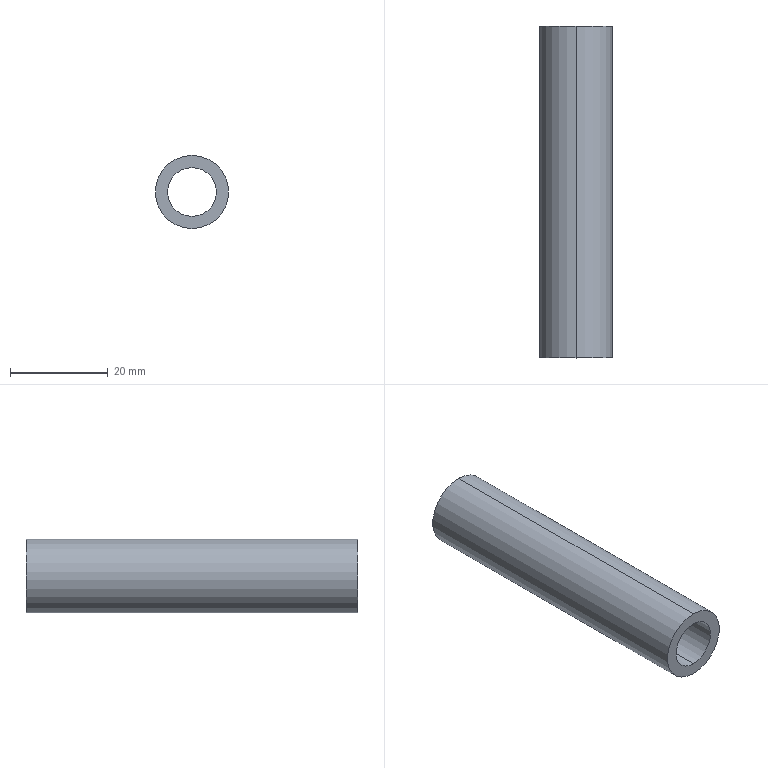Part | STEP file | 1 solid | 6 faces | box 15 x 68 x 15 mm | volume 6676 mm3 | cylinder 4 | plane 2 | commonest cylinder face diameters 10 x2 15 x2
STEP:
#1=CARTESIAN_POINT('',(0.,0.,0.));
#2=DIRECTION('',(0.,0.,1.));
#3=DIRECTION('',(1.,0.,0.));
#4=AXIS2_PLACEMENT_3D('',#1,#2,#3);
#5=CARTESIAN_POINT('',(0.,0.,7.5));
#6=VERTEX_POINT('',#5);
#7=CARTESIAN_POINT('',(0.,0.,-7.5));
#8=VERTEX_POINT('',#7);
#9=CARTESIAN_POINT('',(0.,0.,0.));
#10=DIRECTION('',(0.,1.,0.));
#11=DIRECTION('',(0.,0.,1.));
#12=AXIS2_PLACEMENT_3D('',#9,#10,#11);
#13=CIRCLE('',#12,7.5);
#14=CARTESIAN_POINT('',(0.,0.,0.));
#15=DIRECTION('',(0.,1.,0.));
#16=DIRECTION('',(0.,0.,1.));
#17=AXIS2_PLACEMENT_3D('',#14,#15,#16);
#18=CYLINDRICAL_SURFACE('',#17,7.5);
#19=CARTESIAN_POINT('',(0.,0.));
#20=DIRECTION('',(1.,0.));
#21=VECTOR('',#20,1.);
#22=LINE('',#19,#21);
#23=(GEOMETRIC_REPRESENTATION_CONTEXT(2)PARAMETRIC_REPRESENTATION_CONTEXT()REPRESENTATION_CONTEXT('',''));
#24=DEFINITIONAL_REPRESENTATION('',(#22),#23);
#25=PCURVE('',#18,#24);
#26=CARTESIAN_POINT('',(0.,0.,0.));
#27=DIRECTION('',(0.,1.,0.));
#28=DIRECTION('',(0.,0.,1.));
#29=AXIS2_PLACEMENT_3D('',#26,#27,#28);
#30=PLANE('',#29);
#31=CARTESIAN_POINT('',(0.,0.));
#32=DIRECTION('',(1.,0.));
#33=AXIS2_PLACEMENT_2D('',#31,#32);
#34=CIRCLE('',#33,7.5);
#35=(GEOMETRIC_REPRESENTATION_CONTEXT(2)PARAMETRIC_REPRESENTATION_CONTEXT()REPRESENTATION_CONTEXT('',''));
#36=DEFINITIONAL_REPRESENTATION('',(#34),#35);
#37=PCURVE('',#30,#36);
#38=SURFACE_CURVE('',#13,(#25,#37),.PCURVE_S1.);
#39=EDGE_CURVE('',#6,#8,#38,.T.);
#40=ORIENTED_EDGE('',*,*,#39,.T.);
#41=CARTESIAN_POINT('',(0.,68.,-7.5));
#42=VERTEX_POINT('',#41);
#43=CARTESIAN_POINT('',(0.,0.,-7.5));
#44=DIRECTION('',(0.,1.,0.));
#45=VECTOR('',#44,1.);
#46=LINE('',#43,#45);
#47=CARTESIAN_POINT('',(3.142,0.));
#48=DIRECTION('',(0.,1.));
#49=VECTOR('',#48,1.);
#50=LINE('',#47,#49);
#51=(GEOMETRIC_REPRESENTATION_CONTEXT(2)PARAMETRIC_REPRESENTATION_CONTEXT()REPRESENTATION_CONTEXT('',''));
#52=DEFINITIONAL_REPRESENTATION('',(#50),#51);
#53=PCURVE('',#18,#52);
#54=CARTESIAN_POINT('',(0.,0.,0.));
#55=DIRECTION('',(0.,1.,0.));
#56=DIRECTION('',(0.,0.,1.));
#57=AXIS2_PLACEMENT_3D('',#54,#55,#56);
#58=CYLINDRICAL_SURFACE('',#57,7.5);
#59=CARTESIAN_POINT('',(3.142,0.));
#60=DIRECTION('',(0.,1.));
#61=VECTOR('',#60,1.);
#62=LINE('',#59,#61);
#63=(GEOMETRIC_REPRESENTATION_CONTEXT(2)PARAMETRIC_REPRESENTATION_CONTEXT()REPRESENTATION_CONTEXT('',''));
#64=DEFINITIONAL_REPRESENTATION('',(#62),#63);
#65=PCURVE('',#58,#64);
#66=SURFACE_CURVE('',#46,(#53,#65),.PCURVE_S1.);
#67=EDGE_CURVE('',#8,#42,#66,.T.);
#68=ORIENTED_EDGE('',*,*,#67,.T.);
#69=CARTESIAN_POINT('',(0.,68.,7.5));
#70=VERTEX_POINT('',#69);
#71=CARTESIAN_POINT('',(0.,68.,0.));
#72=DIRECTION('',(0.,-1.,0.));
#73=DIRECTION('',(0.,0.,1.));
#74=AXIS2_PLACEMENT_3D('',#71,#72,#73);
#75=CIRCLE('',#74,7.5);
#76=CARTESIAN_POINT('',(6.283,68.));
#77=DIRECTION('',(-1.,0.));
#78=VECTOR('',#77,1.);
#79=LINE('',#76,#78);
#80=(GEOMETRIC_REPRESENTATION_CONTEXT(2)PARAMETRIC_REPRESENTATION_CONTEXT()REPRESENTATION_CONTEXT('',''));
#81=DEFINITIONAL_REPRESENTATION('',(#79),#80);
#82=PCURVE('',#18,#81);
#83=CARTESIAN_POINT('',(0.,68.,0.));
#84=DIRECTION('',(0.,1.,0.));
#85=DIRECTION('',(0.,0.,1.));
#86=AXIS2_PLACEMENT_3D('',#83,#84,#85);
#87=PLANE('',#86);
#88=CARTESIAN_POINT('',(7.5,0.));
#89=CARTESIAN_POINT('',(7.5,-12.99));
#90=CARTESIAN_POINT('',(-3.75,-6.495));
#91=CARTESIAN_POINT('',(-15.,0.));
#92=CARTESIAN_POINT('',(-3.75,6.495));
#93=CARTESIAN_POINT('',(7.5,12.99));
#94=CARTESIAN_POINT('',(7.5,0.));
#95=(BOUNDED_CURVE()B_SPLINE_CURVE(2,(#88,#89,#90,#91,#92,#93,#94),.UNSPECIFIED.,.T.,.F.)B_SPLINE_CURVE_WITH_KNOTS((1,2,2,2,2,1),(-2.094,0.,2.094,4.189,6.283,8.378),.UNSPECIFIED.)CURVE()GEOMETRIC_REPRESENTATION_ITEM()RATIONAL_B_SPLINE_CURVE((1.,0.5,1.,0.5,1.,0.5,1.))REPRESENTATION_ITEM(''));
#96=(GEOMETRIC_REPRESENTATION_CONTEXT(2)PARAMETRIC_REPRESENTATION_CONTEXT()REPRESENTATION_CONTEXT('',''));
#97=DEFINITIONAL_REPRESENTATION('',(#95),#96);
#98=PCURVE('',#87,#97);
#99=SURFACE_CURVE('',#75,(#82,#98),.PCURVE_S1.);
#100=EDGE_CURVE('',#42,#70,#99,.T.);
#101=ORIENTED_EDGE('',*,*,#100,.T.);
#102=CARTESIAN_POINT('',(0.,0.,7.5));
#103=DIRECTION('',(0.,1.,0.));
#104=VECTOR('',#103,1.);
#105=LINE('',#102,#104);
#106=CARTESIAN_POINT('',(0.,0.));
#107=DIRECTION('',(0.,1.));
#108=VECTOR('',#107,1.);
#109=LINE('',#106,#108);
#110=(GEOMETRIC_REPRESENTATION_CONTEXT(2)PARAMETRIC_REPRESENTATION_CONTEXT()REPRESENTATION_CONTEXT('',''));
#111=DEFINITIONAL_REPRESENTATION('',(#109),#110);
#112=PCURVE('',#18,#111);
#113=CARTESIAN_POINT('',(6.283,0.));
#114=DIRECTION('',(0.,1.));
#115=VECTOR('',#114,1.);
#116=LINE('',#113,#115);
#117=(GEOMETRIC_REPRESENTATION_CONTEXT(2)PARAMETRIC_REPRESENTATION_CONTEXT()REPRESENTATION_CONTEXT('',''));
#118=DEFINITIONAL_REPRESENTATION('',(#116),#117);
#119=PCURVE('',#58,#118);
#120=SURFACE_CURVE('',#105,(#112,#119),.PCURVE_S1.);
#121=EDGE_CURVE('',#6,#70,#120,.T.);
#122=ORIENTED_EDGE('',*,*,#121,.F.);
#123=EDGE_LOOP('',(#40,#68,#101,#122));
#124=FACE_BOUND('',#123,.T.);
#125=ADVANCED_FACE('',(#124),#18,.T.);
#126=CARTESIAN_POINT('',(0.,0.,5.));
#127=VERTEX_POINT('',#126);
#128=CARTESIAN_POINT('',(0.,68.,5.));
#129=VERTEX_POINT('',#128);
#130=CARTESIAN_POINT('',(0.,0.,5.));
#131=DIRECTION('',(0.,1.,0.));
#132=VECTOR('',#131,1.);
#133=LINE('',#130,#132);
#134=CARTESIAN_POINT('',(0.,0.,0.));
#135=DIRECTION('',(0.,1.,0.));
#136=DIRECTION('',(0.,0.,1.));
#137=AXIS2_PLACEMENT_3D('',#134,#135,#136);
#138=CYLINDRICAL_SURFACE('',#137,5.);
#139=CARTESIAN_POINT('',(6.283,0.));
#140=DIRECTION('',(0.,1.));
#141=VECTOR('',#140,1.);
#142=LINE('',#139,#141);
#143=(GEOMETRIC_REPRESENTATION_CONTEXT(2)PARAMETRIC_REPRESENTATION_CONTEXT()REPRESENTATION_CONTEXT('',''));
#144=DEFINITIONAL_REPRESENTATION('',(#142),#143);
#145=PCURVE('',#138,#144);
#146=CARTESIAN_POINT('',(0.,0.,0.));
#147=DIRECTION('',(0.,1.,0.));
#148=DIRECTION('',(0.,0.,1.));
#149=AXIS2_PLACEMENT_3D('',#146,#147,#148);
#150=CYLINDRICAL_SURFACE('',#149,5.);
#151=CARTESIAN_POINT('',(0.,0.));
#152=DIRECTION('',(0.,1.));
#153=VECTOR('',#152,1.);
#154=LINE('',#151,#153);
#155=(GEOMETRIC_REPRESENTATION_CONTEXT(2)PARAMETRIC_REPRESENTATION_CONTEXT()REPRESENTATION_CONTEXT('',''));
#156=DEFINITIONAL_REPRESENTATION('',(#154),#155);
#157=PCURVE('',#150,#156);
#158=SURFACE_CURVE('',#133,(#145,#157),.PCURVE_S1.);
#159=EDGE_CURVE('',#127,#129,#158,.T.);
#160=ORIENTED_EDGE('',*,*,#159,.T.);
#161=CARTESIAN_POINT('',(0.,68.,-5.));
#162=VERTEX_POINT('',#161);
#163=CARTESIAN_POINT('',(0.,68.,0.));
#164=DIRECTION('',(0.,-1.,0.));
#165=DIRECTION('',(0.,0.,1.));
#166=AXIS2_PLACEMENT_3D('',#163,#164,#165);
#167=CIRCLE('',#166,5.);
#168=CARTESIAN_POINT('',(6.283,68.));
#169=DIRECTION('',(-1.,0.));
#170=VECTOR('',#169,1.);
#171=LINE('',#168,#170);
#172=(GEOMETRIC_REPRESENTATION_CONTEXT(2)PARAMETRIC_REPRESENTATION_CONTEXT()REPRESENTATION_CONTEXT('',''));
#173=DEFINITIONAL_REPRESENTATION('',(#171),#172);
#174=PCURVE('',#138,#173);
#175=CARTESIAN_POINT('',(5.,0.));
#176=CARTESIAN_POINT('',(5.,-8.66));
#177=CARTESIAN_POINT('',(-2.5,-4.33));
#178=CARTESIAN_POINT('',(-10.,0.));
#179=CARTESIAN_POINT('',(-2.5,4.33));
#180=CARTESIAN_POINT('',(5.,8.66));
#181=CARTESIAN_POINT('',(5.,0.));
#182=(BOUNDED_CURVE()B_SPLINE_CURVE(2,(#175,#176,#177,#178,#179,#180,#181),.UNSPECIFIED.,.T.,.F.)B_SPLINE_CURVE_WITH_KNOTS((1,2,2,2,2,1),(-2.094,0.,2.094,4.189,6.283,8.378),.UNSPECIFIED.)CURVE()GEOMETRIC_REPRESENTATION_ITEM()RATIONAL_B_SPLINE_CURVE((1.,0.5,1.,0.5,1.,0.5,1.))REPRESENTATION_ITEM(''));
#183=(GEOMETRIC_REPRESENTATION_CONTEXT(2)PARAMETRIC_REPRESENTATION_CONTEXT()REPRESENTATION_CONTEXT('',''));
#184=DEFINITIONAL_REPRESENTATION('',(#182),#183);
#185=PCURVE('',#87,#184);
#186=SURFACE_CURVE('',#167,(#174,#185),.PCURVE_S1.);
#187=EDGE_CURVE('',#129,#162,#186,.T.);
#188=ORIENTED_EDGE('',*,*,#187,.T.);
#189=CARTESIAN_POINT('',(0.,0.,-5.));
#190=VERTEX_POINT('',#189);
#191=CARTESIAN_POINT('',(0.,0.,-5.));
#192=DIRECTION('',(0.,1.,0.));
#193=VECTOR('',#192,1.);
#194=LINE('',#191,#193);
#195=CARTESIAN_POINT('',(3.142,0.));
#196=DIRECTION('',(0.,1.));
#197=VECTOR('',#196,1.);
#198=LINE('',#195,#197);
#199=(GEOMETRIC_REPRESENTATION_CONTEXT(2)PARAMETRIC_REPRESENTATION_CONTEXT()REPRESENTATION_CONTEXT('',''));
#200=DEFINITIONAL_REPRESENTATION('',(#198),#199);
#201=PCURVE('',#138,#200);
#202=CARTESIAN_POINT('',(3.142,0.));
#203=DIRECTION('',(0.,1.));
#204=VECTOR('',#203,1.);
#205=LINE('',#202,#204);
#206=(GEOMETRIC_REPRESENTATION_CONTEXT(2)PARAMETRIC_REPRESENTATION_CONTEXT()REPRESENTATION_CONTEXT('',''));
#207=DEFINITIONAL_REPRESENTATION('',(#205),#206);
#208=PCURVE('',#150,#207);
#209=SURFACE_CURVE('',#194,(#201,#208),.PCURVE_S1.);
#210=EDGE_CURVE('',#190,#162,#209,.T.);
#211=ORIENTED_EDGE('',*,*,#210,.F.);
#212=CARTESIAN_POINT('',(0.,0.,0.));
#213=DIRECTION('',(0.,-1.,0.));
#214=DIRECTION('',(0.,0.,1.));
#215=AXIS2_PLACEMENT_3D('',#212,#213,#214);
#216=CIRCLE('',#215,5.);
#217=CARTESIAN_POINT('',(6.283,0.));
#218=DIRECTION('',(-1.,0.));
#219=VECTOR('',#218,1.);
#220=LINE('',#217,#219);
#221=(GEOMETRIC_REPRESENTATION_CONTEXT(2)PARAMETRIC_REPRESENTATION_CONTEXT()REPRESENTATION_CONTEXT('',''));
#222=DEFINITIONAL_REPRESENTATION('',(#220),#221);
#223=PCURVE('',#138,#222);
#224=CARTESIAN_POINT('',(5.,0.));
#225=CARTESIAN_POINT('',(5.,-8.66));
#226=CARTESIAN_POINT('',(-2.5,-4.33));
#227=CARTESIAN_POINT('',(-10.,0.));
#228=CARTESIAN_POINT('',(-2.5,4.33));
#229=CARTESIAN_POINT('',(5.,8.66));
#230=CARTESIAN_POINT('',(5.,0.));
#231=(BOUNDED_CURVE()B_SPLINE_CURVE(2,(#224,#225,#226,#227,#228,#229,#230),.UNSPECIFIED.,.T.,.F.)B_SPLINE_CURVE_WITH_KNOTS((1,2,2,2,2,1),(-2.094,0.,2.094,4.189,6.283,8.378),.UNSPECIFIED.)CURVE()GEOMETRIC_REPRESENTATION_ITEM()RATIONAL_B_SPLINE_CURVE((1.,0.5,1.,0.5,1.,0.5,1.))REPRESENTATION_ITEM(''));
#232=(GEOMETRIC_REPRESENTATION_CONTEXT(2)PARAMETRIC_REPRESENTATION_CONTEXT()REPRESENTATION_CONTEXT('',''));
#233=DEFINITIONAL_REPRESENTATION('',(#231),#232);
#234=PCURVE('',#30,#233);
#235=SURFACE_CURVE('',#216,(#223,#234),.PCURVE_S1.);
#236=EDGE_CURVE('',#127,#190,#235,.T.);
#237=ORIENTED_EDGE('',*,*,#236,.F.);
#238=EDGE_LOOP('',(#160,#188,#211,#237));
#239=FACE_BOUND('',#238,.F.);
#240=ADVANCED_FACE('',(#239),#138,.F.);
#241=ORIENTED_EDGE('',*,*,#67,.F.);
#242=CARTESIAN_POINT('',(0.,0.,0.));
#243=DIRECTION('',(0.,1.,0.));
#244=DIRECTION('',(0.,0.,1.));
#245=AXIS2_PLACEMENT_3D('',#242,#243,#244);
#246=CIRCLE('',#245,7.5);
#247=CARTESIAN_POINT('',(0.,0.));
#248=DIRECTION('',(1.,0.));
#249=VECTOR('',#248,1.);
#250=LINE('',#247,#249);
#251=(GEOMETRIC_REPRESENTATION_CONTEXT(2)PARAMETRIC_REPRESENTATION_CONTEXT()REPRESENTATION_CONTEXT('',''));
#252=DEFINITIONAL_REPRESENTATION('',(#250),#251);
#253=PCURVE('',#58,#252);
#254=CARTESIAN_POINT('',(0.,0.));
#255=DIRECTION('',(1.,0.));
#256=AXIS2_PLACEMENT_2D('',#254,#255);
#257=CIRCLE('',#256,7.5);
#258=(GEOMETRIC_REPRESENTATION_CONTEXT(2)PARAMETRIC_REPRESENTATION_CONTEXT()REPRESENTATION_CONTEXT('',''));
#259=DEFINITIONAL_REPRESENTATION('',(#257),#258);
#260=PCURVE('',#30,#259);
#261=SURFACE_CURVE('',#246,(#253,#260),.PCURVE_S1.);
#262=EDGE_CURVE('',#8,#6,#261,.T.);
#263=ORIENTED_EDGE('',*,*,#262,.T.);
#264=ORIENTED_EDGE('',*,*,#121,.T.);
#265=CARTESIAN_POINT('',(0.,68.,0.));
#266=DIRECTION('',(0.,-1.,0.));
#267=DIRECTION('',(0.,0.,1.));
#268=AXIS2_PLACEMENT_3D('',#265,#266,#267);
#269=CIRCLE('',#268,7.5);
#270=CARTESIAN_POINT('',(6.283,68.));
#271=DIRECTION('',(-1.,0.));
#272=VECTOR('',#271,1.);
#273=LINE('',#270,#272);
#274=(GEOMETRIC_REPRESENTATION_CONTEXT(2)PARAMETRIC_REPRESENTATION_CONTEXT()REPRESENTATION_CONTEXT('',''));
#275=DEFINITIONAL_REPRESENTATION('',(#273),#274);
#276=PCURVE('',#58,#275);
#277=CARTESIAN_POINT('',(7.5,0.));
#278=CARTESIAN_POINT('',(7.5,-12.99));
#279=CARTESIAN_POINT('',(-3.75,-6.495));
#280=CARTESIAN_POINT('',(-15.,0.));
#281=CARTESIAN_POINT('',(-3.75,6.495));
#282=CARTESIAN_POINT('',(7.5,12.99));
#283=CARTESIAN_POINT('',(7.5,0.));
#284=(BOUNDED_CURVE()B_SPLINE_CURVE(2,(#277,#278,#279,#280,#281,#282,#283),.UNSPECIFIED.,.T.,.F.)B_SPLINE_CURVE_WITH_KNOTS((1,2,2,2,2,1),(-2.094,0.,2.094,4.189,6.283,8.378),.UNSPECIFIED.)CURVE()GEOMETRIC_REPRESENTATION_ITEM()RATIONAL_B_SPLINE_CURVE((1.,0.5,1.,0.5,1.,0.5,1.))REPRESENTATION_ITEM(''));
#285=(GEOMETRIC_REPRESENTATION_CONTEXT(2)PARAMETRIC_REPRESENTATION_CONTEXT()REPRESENTATION_CONTEXT('',''));
#286=DEFINITIONAL_REPRESENTATION('',(#284),#285);
#287=PCURVE('',#87,#286);
#288=SURFACE_CURVE('',#269,(#276,#287),.PCURVE_S1.);
#289=EDGE_CURVE('',#70,#42,#288,.T.);
#290=ORIENTED_EDGE('',*,*,#289,.T.);
#291=EDGE_LOOP('',(#241,#263,#264,#290));
#292=FACE_BOUND('',#291,.T.);
#293=ADVANCED_FACE('',(#292),#58,.T.);
#294=ORIENTED_EDGE('',*,*,#39,.F.);
#295=ORIENTED_EDGE('',*,*,#262,.F.);
#296=EDGE_LOOP('',(#294,#295));
#297=FACE_BOUND('',#296,.T.);
#298=ORIENTED_EDGE('',*,*,#236,.F.);
#299=CARTESIAN_POINT('',(0.,0.,0.));
#300=DIRECTION('',(0.,-1.,0.));
#301=DIRECTION('',(0.,0.,1.));
#302=AXIS2_PLACEMENT_3D('',#299,#300,#301);
#303=CIRCLE('',#302,5.);
#304=CARTESIAN_POINT('',(5.,0.));
#305=CARTESIAN_POINT('',(5.,-8.66));
#306=CARTESIAN_POINT('',(-2.5,-4.33));
#307=CARTESIAN_POINT('',(-10.,0.));
#308=CARTESIAN_POINT('',(-2.5,4.33));
#309=CARTESIAN_POINT('',(5.,8.66));
#310=CARTESIAN_POINT('',(5.,0.));
#311=(BOUNDED_CURVE()B_SPLINE_CURVE(2,(#304,#305,#306,#307,#308,#309,#310),.UNSPECIFIED.,.T.,.F.)B_SPLINE_CURVE_WITH_KNOTS((1,2,2,2,2,1),(-2.094,0.,2.094,4.189,6.283,8.378),.UNSPECIFIED.)CURVE()GEOMETRIC_REPRESENTATION_ITEM()RATIONAL_B_SPLINE_CURVE((1.,0.5,1.,0.5,1.,0.5,1.))REPRESENTATION_ITEM(''));
#312=(GEOMETRIC_REPRESENTATION_CONTEXT(2)PARAMETRIC_REPRESENTATION_CONTEXT()REPRESENTATION_CONTEXT('',''));
#313=DEFINITIONAL_REPRESENTATION('',(#311),#312);
#314=PCURVE('',#30,#313);
#315=CARTESIAN_POINT('',(6.283,0.));
#316=DIRECTION('',(-1.,0.));
#317=VECTOR('',#316,1.);
#318=LINE('',#315,#317);
#319=(GEOMETRIC_REPRESENTATION_CONTEXT(2)PARAMETRIC_REPRESENTATION_CONTEXT()REPRESENTATION_CONTEXT('',''));
#320=DEFINITIONAL_REPRESENTATION('',(#318),#319);
#321=PCURVE('',#150,#320);
#322=SURFACE_CURVE('',#303,(#314,#321),.PCURVE_S1.);
#323=EDGE_CURVE('',#190,#127,#322,.T.);
#324=ORIENTED_EDGE('',*,*,#323,.F.);
#325=EDGE_LOOP('',(#298,#324));
#326=FACE_BOUND('',#325,.T.);
#327=ADVANCED_FACE('',(#297,#326),#30,.F.);
#328=ORIENTED_EDGE('',*,*,#289,.F.);
#329=ORIENTED_EDGE('',*,*,#100,.F.);
#330=EDGE_LOOP('',(#328,#329));
#331=FACE_BOUND('',#330,.T.);
#332=ORIENTED_EDGE('',*,*,#187,.T.);
#333=CARTESIAN_POINT('',(0.,68.,0.));
#334=DIRECTION('',(0.,-1.,0.));
#335=DIRECTION('',(0.,0.,1.));
#336=AXIS2_PLACEMENT_3D('',#333,#334,#335);
#337=CIRCLE('',#336,5.);
#338=CARTESIAN_POINT('',(5.,0.));
#339=CARTESIAN_POINT('',(5.,-8.66));
#340=CARTESIAN_POINT('',(-2.5,-4.33));
#341=CARTESIAN_POINT('',(-10.,0.));
#342=CARTESIAN_POINT('',(-2.5,4.33));
#343=CARTESIAN_POINT('',(5.,8.66));
#344=CARTESIAN_POINT('',(5.,0.));
#345=(BOUNDED_CURVE()B_SPLINE_CURVE(2,(#338,#339,#340,#341,#342,#343,#344),.UNSPECIFIED.,.T.,.F.)B_SPLINE_CURVE_WITH_KNOTS((1,2,2,2,2,1),(-2.094,0.,2.094,4.189,6.283,8.378),.UNSPECIFIED.)CURVE()GEOMETRIC_REPRESENTATION_ITEM()RATIONAL_B_SPLINE_CURVE((1.,0.5,1.,0.5,1.,0.5,1.))REPRESENTATION_ITEM(''));
#346=(GEOMETRIC_REPRESENTATION_CONTEXT(2)PARAMETRIC_REPRESENTATION_CONTEXT()REPRESENTATION_CONTEXT('',''));
#347=DEFINITIONAL_REPRESENTATION('',(#345),#346);
#348=PCURVE('',#87,#347);
#349=CARTESIAN_POINT('',(6.283,68.));
#350=DIRECTION('',(-1.,0.));
#351=VECTOR('',#350,1.);
#352=LINE('',#349,#351);
#353=(GEOMETRIC_REPRESENTATION_CONTEXT(2)PARAMETRIC_REPRESENTATION_CONTEXT()REPRESENTATION_CONTEXT('',''));
#354=DEFINITIONAL_REPRESENTATION('',(#352),#353);
#355=PCURVE('',#150,#354);
#356=SURFACE_CURVE('',#337,(#348,#355),.PCURVE_S1.);
#357=EDGE_CURVE('',#162,#129,#356,.T.);
#358=ORIENTED_EDGE('',*,*,#357,.T.);
#359=EDGE_LOOP('',(#332,#358));
#360=FACE_BOUND('',#359,.T.);
#361=ADVANCED_FACE('',(#331,#360),#87,.T.);
#362=ORIENTED_EDGE('',*,*,#357,.T.);
#363=ORIENTED_EDGE('',*,*,#159,.F.);
#364=ORIENTED_EDGE('',*,*,#323,.F.);
#365=ORIENTED_EDGE('',*,*,#210,.T.);
#366=EDGE_LOOP('',(#362,#363,#364,#365));
#367=FACE_BOUND('',#366,.F.);
#368=ADVANCED_FACE('',(#367),#150,.F.);
#369=CLOSED_SHELL('',(#125,#240,#293,#327,#361,#368));
#370=MANIFOLD_SOLID_BREP('',#369);
#371=(LENGTH_UNIT()NAMED_UNIT(*)SI_UNIT(.MILLI.,.METRE.));
#372=UNCERTAINTY_MEASURE_WITH_UNIT(LENGTH_MEASURE(0.0000001),#371,'','');
#373=(NAMED_UNIT(*)PLANE_ANGLE_UNIT()SI_UNIT($,.RADIAN.));
#374=(NAMED_UNIT(*)SI_UNIT($,.STERADIAN.)SOLID_ANGLE_UNIT());
#375=(GEOMETRIC_REPRESENTATION_CONTEXT(3)GLOBAL_UNCERTAINTY_ASSIGNED_CONTEXT((#372))GLOBAL_UNIT_ASSIGNED_CONTEXT((#371,#373,#374))REPRESENTATION_CONTEXT('',''));
#376=ADVANCED_BREP_SHAPE_REPRESENTATION('',(#4,#370),#375);